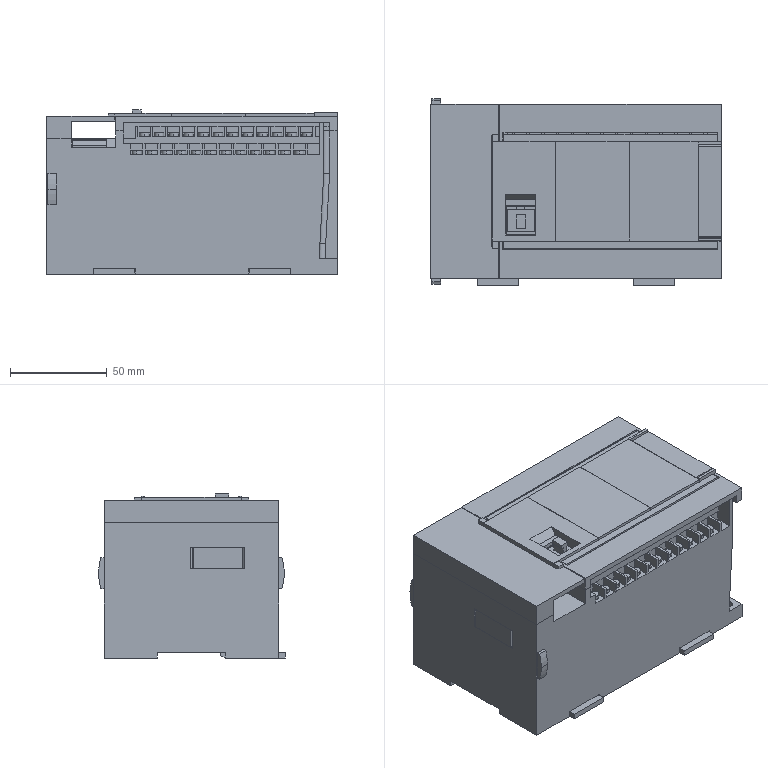Part | STEP file | PLC module FX5U-32MT_ES | 14 solids | 1200 faces | box 150 x 96.4 x 84.9 mm | volume 980252 mm3 | plane 887 | cylinder 310 | cone 3 | commonest cylinder face diameters 5 x96 1.8 x84 1.6 x81 6 x9 4 x7 4.5 x6